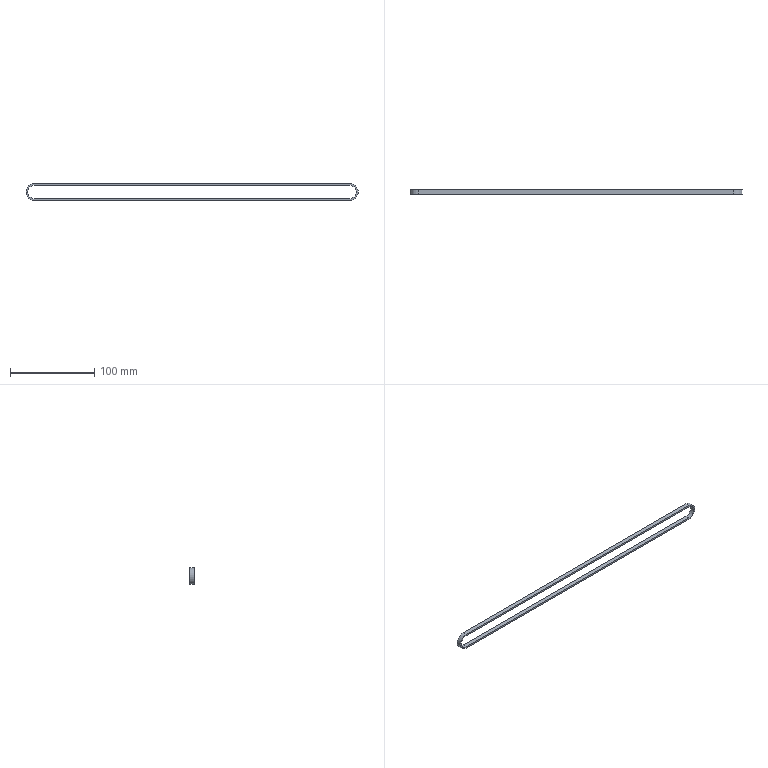Part | SolidWorks | features Extrusion 1 | 1 solid | 10 faces | box 395 x 5 x 20 mm | volume 8065 mm3 | plane 6 | cylinder 4 | commonest cylinder face diameters 16 x2 20 x2
STEP:
#1=CARTESIAN_POINT('',(-348.959,5.,-10.));
#2=VERTEX_POINT('',#1);
#3=CARTESIAN_POINT('',(-348.959,5.,10.));
#4=VERTEX_POINT('',#3);
#5=CARTESIAN_POINT('',(-348.959,5.,0.));
#6=DIRECTION('',(0.,1.,0.));
#7=DIRECTION('',(0.,0.,1.));
#8=AXIS2_PLACEMENT_3D('',#5,#6,#7);
#9=CIRCLE('',#8,10.);
#10=EDGE_CURVE('',#2,#4,#9,.T.);
#11=ORIENTED_EDGE('',*,*,#10,.T.);
#12=CARTESIAN_POINT('',(26.041,5.,10.));
#13=VERTEX_POINT('',#12);
#14=CARTESIAN_POINT('',(-348.959,5.,10.));
#15=DIRECTION('',(1.,0.,0.));
#16=VECTOR('',#15,1000.);
#17=LINE('',#14,#16);
#18=EDGE_CURVE('',#4,#13,#17,.T.);
#19=ORIENTED_EDGE('',*,*,#18,.T.);
#20=CARTESIAN_POINT('',(26.041,5.,-10.));
#21=VERTEX_POINT('',#20);
#22=CARTESIAN_POINT('',(26.041,5.,0.));
#23=DIRECTION('',(0.,1.,0.));
#24=DIRECTION('',(0.,0.,1.));
#25=AXIS2_PLACEMENT_3D('',#22,#23,#24);
#26=CIRCLE('',#25,10.);
#27=EDGE_CURVE('',#13,#21,#26,.T.);
#28=ORIENTED_EDGE('',*,*,#27,.T.);
#29=CARTESIAN_POINT('',(-348.959,5.,-10.));
#30=DIRECTION('',(-1.,0.,0.));
#31=VECTOR('',#30,1000.);
#32=LINE('',#29,#31);
#33=EDGE_CURVE('',#21,#2,#32,.T.);
#34=ORIENTED_EDGE('',*,*,#33,.T.);
#35=EDGE_LOOP('',(#11,#19,#28,#34));
#36=FACE_OUTER_BOUND('',#35,.T.);
#37=CARTESIAN_POINT('',(-348.959,5.,8.));
#38=VERTEX_POINT('',#37);
#39=CARTESIAN_POINT('',(26.041,5.,8.));
#40=VERTEX_POINT('',#39);
#41=CARTESIAN_POINT('',(-348.959,5.,8.));
#42=DIRECTION('',(1.,0.,0.));
#43=VECTOR('',#42,1000.);
#44=LINE('',#41,#43);
#45=EDGE_CURVE('',#38,#40,#44,.T.);
#46=ORIENTED_EDGE('',*,*,#45,.F.);
#47=CARTESIAN_POINT('',(-348.959,5.,-8.));
#48=VERTEX_POINT('',#47);
#49=CARTESIAN_POINT('',(-348.959,5.,0.));
#50=DIRECTION('',(0.,1.,0.));
#51=DIRECTION('',(0.,0.,1.));
#52=AXIS2_PLACEMENT_3D('',#49,#50,#51);
#53=CIRCLE('',#52,8.);
#54=EDGE_CURVE('',#48,#38,#53,.T.);
#55=ORIENTED_EDGE('',*,*,#54,.F.);
#56=CARTESIAN_POINT('',(26.041,5.,-8.));
#57=VERTEX_POINT('',#56);
#58=CARTESIAN_POINT('',(-348.959,5.,-8.));
#59=DIRECTION('',(-1.,0.,0.));
#60=VECTOR('',#59,1000.);
#61=LINE('',#58,#60);
#62=EDGE_CURVE('',#57,#48,#61,.T.);
#63=ORIENTED_EDGE('',*,*,#62,.F.);
#64=CARTESIAN_POINT('',(26.041,5.,0.));
#65=DIRECTION('',(0.,1.,0.));
#66=DIRECTION('',(0.,0.,1.));
#67=AXIS2_PLACEMENT_3D('',#64,#65,#66);
#68=CIRCLE('',#67,8.);
#69=EDGE_CURVE('',#40,#57,#68,.T.);
#70=ORIENTED_EDGE('',*,*,#69,.F.);
#71=EDGE_LOOP('',(#46,#55,#63,#70));
#72=FACE_BOUND('',#71,.T.);
#73=CARTESIAN_POINT('',(-348.959,5.,0.));
#74=DIRECTION('',(0.,1.,0.));
#75=DIRECTION('',(0.,0.,1.));
#76=AXIS2_PLACEMENT_3D('',#73,#74,#75);
#77=PLANE('',#76);
#78=ADVANCED_FACE('',(#36,#72),#77,.T.);
#79=CARTESIAN_POINT('',(-348.959,0.,-10.));
#80=VERTEX_POINT('',#79);
#81=CARTESIAN_POINT('',(-348.959,0.,10.));
#82=VERTEX_POINT('',#81);
#83=CARTESIAN_POINT('',(-348.959,0.,0.));
#84=DIRECTION('',(0.,1.,0.));
#85=DIRECTION('',(0.,0.,1.));
#86=AXIS2_PLACEMENT_3D('',#83,#84,#85);
#87=CIRCLE('',#86,10.);
#88=EDGE_CURVE('',#80,#82,#87,.T.);
#89=ORIENTED_EDGE('',*,*,#88,.F.);
#90=CARTESIAN_POINT('',(26.041,0.,-10.));
#91=VERTEX_POINT('',#90);
#92=CARTESIAN_POINT('',(-348.959,0.,-10.));
#93=DIRECTION('',(-1.,0.,0.));
#94=VECTOR('',#93,1000.);
#95=LINE('',#92,#94);
#96=EDGE_CURVE('',#91,#80,#95,.T.);
#97=ORIENTED_EDGE('',*,*,#96,.F.);
#98=CARTESIAN_POINT('',(26.041,0.,10.));
#99=VERTEX_POINT('',#98);
#100=CARTESIAN_POINT('',(26.041,0.,0.));
#101=DIRECTION('',(0.,1.,0.));
#102=DIRECTION('',(0.,0.,1.));
#103=AXIS2_PLACEMENT_3D('',#100,#101,#102);
#104=CIRCLE('',#103,10.);
#105=EDGE_CURVE('',#99,#91,#104,.T.);
#106=ORIENTED_EDGE('',*,*,#105,.F.);
#107=CARTESIAN_POINT('',(-348.959,0.,10.));
#108=DIRECTION('',(1.,0.,0.));
#109=VECTOR('',#108,1000.);
#110=LINE('',#107,#109);
#111=EDGE_CURVE('',#82,#99,#110,.T.);
#112=ORIENTED_EDGE('',*,*,#111,.F.);
#113=EDGE_LOOP('',(#89,#97,#106,#112));
#114=FACE_OUTER_BOUND('',#113,.T.);
#115=CARTESIAN_POINT('',(-348.959,0.,-8.));
#116=VERTEX_POINT('',#115);
#117=CARTESIAN_POINT('',(-348.959,0.,8.));
#118=VERTEX_POINT('',#117);
#119=CARTESIAN_POINT('',(-348.959,0.,0.));
#120=DIRECTION('',(0.,1.,0.));
#121=DIRECTION('',(0.,0.,1.));
#122=AXIS2_PLACEMENT_3D('',#119,#120,#121);
#123=CIRCLE('',#122,8.);
#124=EDGE_CURVE('',#116,#118,#123,.T.);
#125=ORIENTED_EDGE('',*,*,#124,.T.);
#126=CARTESIAN_POINT('',(26.041,0.,8.));
#127=VERTEX_POINT('',#126);
#128=CARTESIAN_POINT('',(-348.959,0.,8.));
#129=DIRECTION('',(1.,0.,0.));
#130=VECTOR('',#129,1000.);
#131=LINE('',#128,#130);
#132=EDGE_CURVE('',#118,#127,#131,.T.);
#133=ORIENTED_EDGE('',*,*,#132,.T.);
#134=CARTESIAN_POINT('',(26.041,0.,-8.));
#135=VERTEX_POINT('',#134);
#136=CARTESIAN_POINT('',(26.041,0.,0.));
#137=DIRECTION('',(0.,1.,0.));
#138=DIRECTION('',(0.,0.,1.));
#139=AXIS2_PLACEMENT_3D('',#136,#137,#138);
#140=CIRCLE('',#139,8.);
#141=EDGE_CURVE('',#127,#135,#140,.T.);
#142=ORIENTED_EDGE('',*,*,#141,.T.);
#143=CARTESIAN_POINT('',(-348.959,0.,-8.));
#144=DIRECTION('',(-1.,0.,0.));
#145=VECTOR('',#144,1000.);
#146=LINE('',#143,#145);
#147=EDGE_CURVE('',#135,#116,#146,.T.);
#148=ORIENTED_EDGE('',*,*,#147,.T.);
#149=EDGE_LOOP('',(#125,#133,#142,#148));
#150=FACE_BOUND('',#149,.T.);
#151=CARTESIAN_POINT('',(-348.959,0.,0.));
#152=DIRECTION('',(0.,1.,0.));
#153=DIRECTION('',(0.,0.,1.));
#154=AXIS2_PLACEMENT_3D('',#151,#152,#153);
#155=PLANE('',#154);
#156=ADVANCED_FACE('',(#114,#150),#155,.F.);
#157=ORIENTED_EDGE('',*,*,#88,.T.);
#158=CARTESIAN_POINT('',(-348.959,5.,10.));
#159=DIRECTION('',(0.,-1.,0.));
#160=VECTOR('',#159,1000.);
#161=LINE('',#158,#160);
#162=EDGE_CURVE('',#4,#82,#161,.T.);
#163=ORIENTED_EDGE('',*,*,#162,.F.);
#164=ORIENTED_EDGE('',*,*,#10,.F.);
#165=CARTESIAN_POINT('',(-348.959,5.,-10.));
#166=DIRECTION('',(0.,-1.,0.));
#167=VECTOR('',#166,1000.);
#168=LINE('',#165,#167);
#169=EDGE_CURVE('',#2,#80,#168,.T.);
#170=ORIENTED_EDGE('',*,*,#169,.T.);
#171=EDGE_LOOP('',(#157,#163,#164,#170));
#172=FACE_OUTER_BOUND('',#171,.T.);
#173=CARTESIAN_POINT('',(-348.959,5.,0.));
#174=DIRECTION('',(0.,-1.,0.));
#175=DIRECTION('',(0.,0.,-1.));
#176=AXIS2_PLACEMENT_3D('',#173,#174,#175);
#177=CYLINDRICAL_SURFACE('',#176,10.);
#178=ADVANCED_FACE('',(#172),#177,.T.);
#179=ORIENTED_EDGE('',*,*,#111,.T.);
#180=CARTESIAN_POINT('',(26.041,5.,10.));
#181=DIRECTION('',(0.,-1.,0.));
#182=VECTOR('',#181,1000.);
#183=LINE('',#180,#182);
#184=EDGE_CURVE('',#13,#99,#183,.T.);
#185=ORIENTED_EDGE('',*,*,#184,.F.);
#186=ORIENTED_EDGE('',*,*,#18,.F.);
#187=ORIENTED_EDGE('',*,*,#162,.T.);
#188=EDGE_LOOP('',(#179,#185,#186,#187));
#189=FACE_OUTER_BOUND('',#188,.T.);
#190=CARTESIAN_POINT('',(-348.959,5.,10.));
#191=DIRECTION('',(0.,0.,-1.));
#192=DIRECTION('',(-1.,0.,0.));
#193=AXIS2_PLACEMENT_3D('',#190,#191,#192);
#194=PLANE('',#193);
#195=ADVANCED_FACE('',(#189),#194,.F.);
#196=ORIENTED_EDGE('',*,*,#105,.T.);
#197=CARTESIAN_POINT('',(26.041,5.,-10.));
#198=DIRECTION('',(0.,-1.,0.));
#199=VECTOR('',#198,1000.);
#200=LINE('',#197,#199);
#201=EDGE_CURVE('',#21,#91,#200,.T.);
#202=ORIENTED_EDGE('',*,*,#201,.F.);
#203=ORIENTED_EDGE('',*,*,#27,.F.);
#204=ORIENTED_EDGE('',*,*,#184,.T.);
#205=EDGE_LOOP('',(#196,#202,#203,#204));
#206=FACE_OUTER_BOUND('',#205,.T.);
#207=CARTESIAN_POINT('',(26.041,5.,0.));
#208=DIRECTION('',(0.,-1.,0.));
#209=DIRECTION('',(0.,0.,-1.));
#210=AXIS2_PLACEMENT_3D('',#207,#208,#209);
#211=CYLINDRICAL_SURFACE('',#210,10.);
#212=ADVANCED_FACE('',(#206),#211,.T.);
#213=ORIENTED_EDGE('',*,*,#96,.T.);
#214=ORIENTED_EDGE('',*,*,#169,.F.);
#215=ORIENTED_EDGE('',*,*,#33,.F.);
#216=ORIENTED_EDGE('',*,*,#201,.T.);
#217=EDGE_LOOP('',(#213,#214,#215,#216));
#218=FACE_OUTER_BOUND('',#217,.T.);
#219=CARTESIAN_POINT('',(-348.959,5.,-10.));
#220=DIRECTION('',(0.,0.,1.));
#221=DIRECTION('',(1.,0.,0.));
#222=AXIS2_PLACEMENT_3D('',#219,#220,#221);
#223=PLANE('',#222);
#224=ADVANCED_FACE('',(#218),#223,.F.);
#225=ORIENTED_EDGE('',*,*,#124,.F.);
#226=CARTESIAN_POINT('',(-348.959,5.,-8.));
#227=DIRECTION('',(0.,-1.,0.));
#228=VECTOR('',#227,1000.);
#229=LINE('',#226,#228);
#230=EDGE_CURVE('',#48,#116,#229,.T.);
#231=ORIENTED_EDGE('',*,*,#230,.F.);
#232=ORIENTED_EDGE('',*,*,#54,.T.);
#233=CARTESIAN_POINT('',(-348.959,5.,8.));
#234=DIRECTION('',(0.,-1.,0.));
#235=VECTOR('',#234,1000.);
#236=LINE('',#233,#235);
#237=EDGE_CURVE('',#38,#118,#236,.T.);
#238=ORIENTED_EDGE('',*,*,#237,.T.);
#239=EDGE_LOOP('',(#225,#231,#232,#238));
#240=FACE_OUTER_BOUND('',#239,.T.);
#241=CARTESIAN_POINT('',(-348.959,5.,0.));
#242=DIRECTION('',(0.,-1.,0.));
#243=DIRECTION('',(0.,0.,-1.));
#244=AXIS2_PLACEMENT_3D('',#241,#242,#243);
#245=CYLINDRICAL_SURFACE('',#244,8.);
#246=ADVANCED_FACE('',(#240),#245,.F.);
#247=ORIENTED_EDGE('',*,*,#132,.F.);
#248=ORIENTED_EDGE('',*,*,#237,.F.);
#249=ORIENTED_EDGE('',*,*,#45,.T.);
#250=CARTESIAN_POINT('',(26.041,5.,8.));
#251=DIRECTION('',(0.,-1.,0.));
#252=VECTOR('',#251,1000.);
#253=LINE('',#250,#252);
#254=EDGE_CURVE('',#40,#127,#253,.T.);
#255=ORIENTED_EDGE('',*,*,#254,.T.);
#256=EDGE_LOOP('',(#247,#248,#249,#255));
#257=FACE_OUTER_BOUND('',#256,.T.);
#258=CARTESIAN_POINT('',(-348.959,5.,8.));
#259=DIRECTION('',(0.,0.,-1.));
#260=DIRECTION('',(-1.,0.,0.));
#261=AXIS2_PLACEMENT_3D('',#258,#259,#260);
#262=PLANE('',#261);
#263=ADVANCED_FACE('',(#257),#262,.T.);
#264=ORIENTED_EDGE('',*,*,#141,.F.);
#265=ORIENTED_EDGE('',*,*,#254,.F.);
#266=ORIENTED_EDGE('',*,*,#69,.T.);
#267=CARTESIAN_POINT('',(26.041,5.,-8.));
#268=DIRECTION('',(0.,-1.,0.));
#269=VECTOR('',#268,1000.);
#270=LINE('',#267,#269);
#271=EDGE_CURVE('',#57,#135,#270,.T.);
#272=ORIENTED_EDGE('',*,*,#271,.T.);
#273=EDGE_LOOP('',(#264,#265,#266,#272));
#274=FACE_OUTER_BOUND('',#273,.T.);
#275=CARTESIAN_POINT('',(26.041,5.,0.));
#276=DIRECTION('',(0.,-1.,0.));
#277=DIRECTION('',(0.,0.,-1.));
#278=AXIS2_PLACEMENT_3D('',#275,#276,#277);
#279=CYLINDRICAL_SURFACE('',#278,8.);
#280=ADVANCED_FACE('',(#274),#279,.F.);
#281=ORIENTED_EDGE('',*,*,#147,.F.);
#282=ORIENTED_EDGE('',*,*,#271,.F.);
#283=ORIENTED_EDGE('',*,*,#62,.T.);
#284=ORIENTED_EDGE('',*,*,#230,.T.);
#285=EDGE_LOOP('',(#281,#282,#283,#284));
#286=FACE_OUTER_BOUND('',#285,.T.);
#287=CARTESIAN_POINT('',(-348.959,5.,-8.));
#288=DIRECTION('',(0.,0.,1.));
#289=DIRECTION('',(1.,0.,0.));
#290=AXIS2_PLACEMENT_3D('',#287,#288,#289);
#291=PLANE('',#290);
#292=ADVANCED_FACE('',(#286),#291,.T.);
#293=CLOSED_SHELL('',(#78,#156,#178,#195,#212,#224,#246,#263,#280,#292));
#294=MANIFOLD_SOLID_BREP('',#293);
#295=CARTESIAN_POINT('',(0.,0.,0.));
#296=DIRECTION('',(0.,0.,1.));
#297=DIRECTION('',(1.,0.,0.));
#298=AXIS2_PLACEMENT_3D('',#295,#296,#297);
#299=(LENGTH_UNIT()NAMED_UNIT(*)SI_UNIT(.MILLI.,.METRE.));
#300=UNCERTAINTY_MEASURE_WITH_UNIT(LENGTH_MEASURE(0.00001),#299,'','');
#301=(NAMED_UNIT(*)PLANE_ANGLE_UNIT()SI_UNIT($,.RADIAN.));
#302=(NAMED_UNIT(*)SI_UNIT($,.STERADIAN.)SOLID_ANGLE_UNIT());
#303=(GEOMETRIC_REPRESENTATION_CONTEXT(3)GLOBAL_UNCERTAINTY_ASSIGNED_CONTEXT((#300))GLOBAL_UNIT_ASSIGNED_CONTEXT((#299,#301,#302))REPRESENTATION_CONTEXT('',''));
#304=ADVANCED_BREP_SHAPE_REPRESENTATION('',(#294,#298),#303);